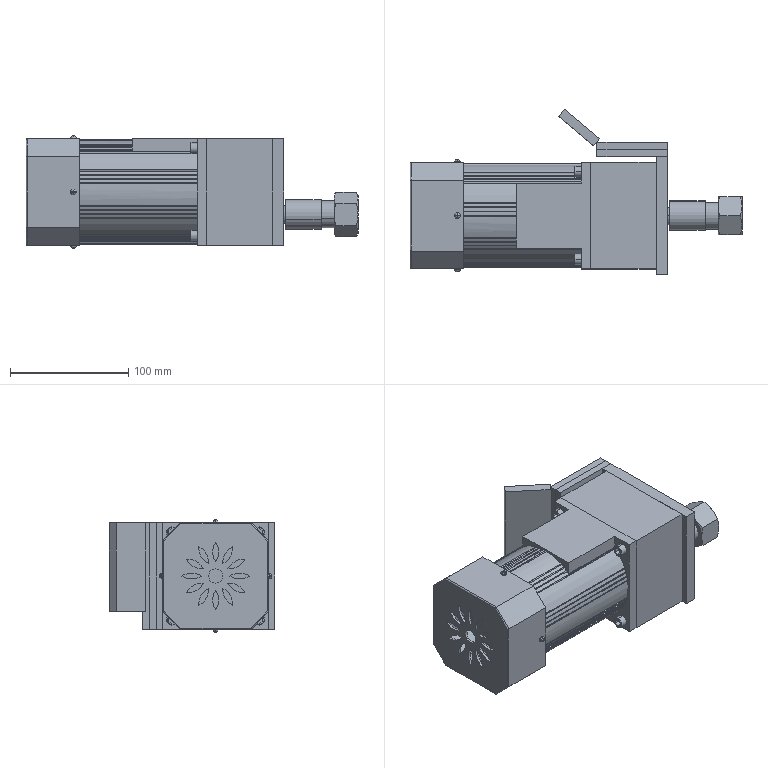Part | SolidWorks | 14 solids | 435 faces | box 280.7 x 140.048 x 94.951 mm | volume 1394120 mm3 | plane 206 | cylinder 185 | cone 28 | sphere 8 | torus 8 | commonest cylinder face diameters 1.5 x44 87 x36 30 x30 5 x17 6 x16 15 x12